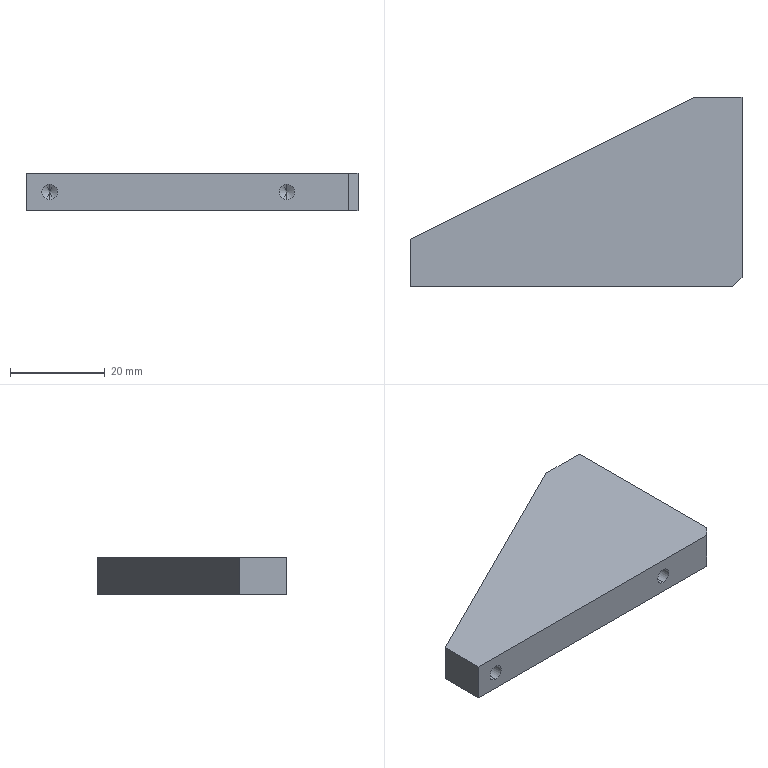Part | SolidWorks | features HoleWzd 2, Chamfer 1, Extrusion 1 | 1 solid | 24 faces | box 70 x 40 x 8 mm | volume 14827 mm3 | cylinder 8 | cone 8 | plane 8 | commonest cylinder face diameters 3.3 x8
STEP:
#1=CARTESIAN_POINT('',(-10.1,35.,5.65));
#2=VERTEX_POINT('',#1);
#3=CARTESIAN_POINT('',(-10.1,35.,2.35));
#4=VERTEX_POINT('',#3);
#5=CARTESIAN_POINT('',(-10.1,35.,4.));
#6=DIRECTION('',(1.,0.,0.));
#7=DIRECTION('',(0.,0.,-1.));
#8=AXIS2_PLACEMENT_3D('',#5,#6,#7);
#9=CIRCLE('',#8,1.65);
#10=EDGE_CURVE('',#2,#4,#9,.T.);
#11=ORIENTED_EDGE('',*,*,#10,.F.);
#12=CARTESIAN_POINT('',(0.,35.,5.65));
#13=VERTEX_POINT('',#12);
#14=CARTESIAN_POINT('',(0.,35.,5.65));
#15=DIRECTION('',(1.,0.,0.));
#16=VECTOR('',#15,1000.);
#17=LINE('',#14,#16);
#18=EDGE_CURVE('',#2,#13,#17,.T.);
#19=ORIENTED_EDGE('',*,*,#18,.T.);
#20=CARTESIAN_POINT('',(0.,35.,2.35));
#21=VERTEX_POINT('',#20);
#22=CARTESIAN_POINT('',(0.,35.,4.));
#23=DIRECTION('',(1.,0.,0.));
#24=DIRECTION('',(0.,0.,-1.));
#25=AXIS2_PLACEMENT_3D('',#22,#23,#24);
#26=CIRCLE('',#25,1.65);
#27=EDGE_CURVE('',#13,#21,#26,.T.);
#28=ORIENTED_EDGE('',*,*,#27,.T.);
#29=CARTESIAN_POINT('',(0.,35.,2.35));
#30=DIRECTION('',(1.,0.,0.));
#31=VECTOR('',#30,1000.);
#32=LINE('',#29,#31);
#33=EDGE_CURVE('',#4,#21,#32,.T.);
#34=ORIENTED_EDGE('',*,*,#33,.F.);
#35=EDGE_LOOP('',(#11,#19,#28,#34));
#36=FACE_OUTER_BOUND('',#35,.T.);
#37=CARTESIAN_POINT('',(0.,35.,4.));
#38=DIRECTION('',(1.,0.,0.));
#39=DIRECTION('',(0.,0.,-1.));
#40=AXIS2_PLACEMENT_3D('',#37,#38,#39);
#41=CYLINDRICAL_SURFACE('',#40,1.65);
#42=ADVANCED_FACE('',(#36),#41,.F.);
#43=CARTESIAN_POINT('',(-11.091,35.,4.));
#44=VERTEX_POINT('',#43);
#45=CARTESIAN_POINT('',(-10.1,35.,2.35));
#46=DIRECTION('',(0.515,0.,-0.8572));
#47=VECTOR('',#46,1000.);
#48=LINE('',#45,#47);
#49=EDGE_CURVE('',#44,#4,#48,.T.);
#50=ORIENTED_EDGE('',*,*,#49,.F.);
#51=CARTESIAN_POINT('',(-10.1,35.,5.65));
#52=DIRECTION('',(0.515,0.,0.8572));
#53=VECTOR('',#52,1000.);
#54=LINE('',#51,#53);
#55=EDGE_CURVE('',#44,#2,#54,.T.);
#56=ORIENTED_EDGE('',*,*,#55,.T.);
#57=ORIENTED_EDGE('',*,*,#10,.T.);
#58=EDGE_LOOP('',(#50,#56,#57));
#59=FACE_OUTER_BOUND('',#58,.T.);
#60=CARTESIAN_POINT('',(-10.1,35.,4.));
#61=DIRECTION('',(1.,0.,0.));
#62=DIRECTION('',(0.,0.,-1.));
#63=AXIS2_PLACEMENT_3D('',#60,#61,#62);
#64=CONICAL_SURFACE('',#63,1.65,1.03);
#65=ADVANCED_FACE('',(#59),#64,.F.);
#66=CARTESIAN_POINT('',(-10.1,15.,5.65));
#67=VERTEX_POINT('',#66);
#68=CARTESIAN_POINT('',(-10.1,15.,2.35));
#69=VERTEX_POINT('',#68);
#70=CARTESIAN_POINT('',(-10.1,15.,4.));
#71=DIRECTION('',(1.,0.,0.));
#72=DIRECTION('',(0.,0.,-1.));
#73=AXIS2_PLACEMENT_3D('',#70,#71,#72);
#74=CIRCLE('',#73,1.65);
#75=EDGE_CURVE('',#67,#69,#74,.T.);
#76=ORIENTED_EDGE('',*,*,#75,.F.);
#77=CARTESIAN_POINT('',(0.,15.,5.65));
#78=VERTEX_POINT('',#77);
#79=CARTESIAN_POINT('',(0.,15.,5.65));
#80=DIRECTION('',(1.,0.,0.));
#81=VECTOR('',#80,1000.);
#82=LINE('',#79,#81);
#83=EDGE_CURVE('',#67,#78,#82,.T.);
#84=ORIENTED_EDGE('',*,*,#83,.T.);
#85=CARTESIAN_POINT('',(0.,15.,2.35));
#86=VERTEX_POINT('',#85);
#87=CARTESIAN_POINT('',(0.,15.,4.));
#88=DIRECTION('',(1.,0.,0.));
#89=DIRECTION('',(0.,0.,-1.));
#90=AXIS2_PLACEMENT_3D('',#87,#88,#89);
#91=CIRCLE('',#90,1.65);
#92=EDGE_CURVE('',#78,#86,#91,.T.);
#93=ORIENTED_EDGE('',*,*,#92,.T.);
#94=CARTESIAN_POINT('',(0.,15.,2.35));
#95=DIRECTION('',(1.,0.,0.));
#96=VECTOR('',#95,1000.);
#97=LINE('',#94,#96);
#98=EDGE_CURVE('',#69,#86,#97,.T.);
#99=ORIENTED_EDGE('',*,*,#98,.F.);
#100=EDGE_LOOP('',(#76,#84,#93,#99));
#101=FACE_OUTER_BOUND('',#100,.T.);
#102=CARTESIAN_POINT('',(0.,15.,4.));
#103=DIRECTION('',(1.,0.,0.));
#104=DIRECTION('',(0.,0.,-1.));
#105=AXIS2_PLACEMENT_3D('',#102,#103,#104);
#106=CYLINDRICAL_SURFACE('',#105,1.65);
#107=ADVANCED_FACE('',(#101),#106,.F.);
#108=CARTESIAN_POINT('',(-11.091,15.,4.));
#109=VERTEX_POINT('',#108);
#110=CARTESIAN_POINT('',(-10.1,15.,2.35));
#111=DIRECTION('',(0.515,0.,-0.8572));
#112=VECTOR('',#111,1000.);
#113=LINE('',#110,#112);
#114=EDGE_CURVE('',#109,#69,#113,.T.);
#115=ORIENTED_EDGE('',*,*,#114,.F.);
#116=CARTESIAN_POINT('',(-10.1,15.,5.65));
#117=DIRECTION('',(0.515,0.,0.8572));
#118=VECTOR('',#117,1000.);
#119=LINE('',#116,#118);
#120=EDGE_CURVE('',#109,#67,#119,.T.);
#121=ORIENTED_EDGE('',*,*,#120,.T.);
#122=ORIENTED_EDGE('',*,*,#75,.T.);
#123=EDGE_LOOP('',(#115,#121,#122));
#124=FACE_OUTER_BOUND('',#123,.T.);
#125=CARTESIAN_POINT('',(-10.1,15.,4.));
#126=DIRECTION('',(1.,0.,0.));
#127=DIRECTION('',(0.,0.,-1.));
#128=AXIS2_PLACEMENT_3D('',#125,#126,#127);
#129=CONICAL_SURFACE('',#128,1.65,1.03);
#130=ADVANCED_FACE('',(#124),#129,.F.);
#131=CARTESIAN_POINT('',(-15.,10.1,5.65));
#132=VERTEX_POINT('',#131);
#133=CARTESIAN_POINT('',(-15.,10.1,2.35));
#134=VERTEX_POINT('',#133);
#135=CARTESIAN_POINT('',(-15.,10.1,4.));
#136=DIRECTION('',(0.,-1.,0.));
#137=DIRECTION('',(0.,0.,-1.));
#138=AXIS2_PLACEMENT_3D('',#135,#136,#137);
#139=CIRCLE('',#138,1.65);
#140=EDGE_CURVE('',#132,#134,#139,.T.);
#141=ORIENTED_EDGE('',*,*,#140,.F.);
#142=CARTESIAN_POINT('',(-15.,0.,5.65));
#143=VERTEX_POINT('',#142);
#144=CARTESIAN_POINT('',(-15.,0.,5.65));
#145=DIRECTION('',(0.,-1.,0.));
#146=VECTOR('',#145,1000.);
#147=LINE('',#144,#146);
#148=EDGE_CURVE('',#132,#143,#147,.T.);
#149=ORIENTED_EDGE('',*,*,#148,.T.);
#150=CARTESIAN_POINT('',(-15.,0.,2.35));
#151=VERTEX_POINT('',#150);
#152=CARTESIAN_POINT('',(-15.,0.,4.));
#153=DIRECTION('',(0.,-1.,0.));
#154=DIRECTION('',(0.,0.,-1.));
#155=AXIS2_PLACEMENT_3D('',#152,#153,#154);
#156=CIRCLE('',#155,1.65);
#157=EDGE_CURVE('',#143,#151,#156,.T.);
#158=ORIENTED_EDGE('',*,*,#157,.T.);
#159=CARTESIAN_POINT('',(-15.,0.,2.35));
#160=DIRECTION('',(0.,-1.,0.));
#161=VECTOR('',#160,1000.);
#162=LINE('',#159,#161);
#163=EDGE_CURVE('',#134,#151,#162,.T.);
#164=ORIENTED_EDGE('',*,*,#163,.F.);
#165=EDGE_LOOP('',(#141,#149,#158,#164));
#166=FACE_OUTER_BOUND('',#165,.T.);
#167=CARTESIAN_POINT('',(-15.,0.,4.));
#168=DIRECTION('',(0.,-1.,0.));
#169=DIRECTION('',(0.,0.,-1.));
#170=AXIS2_PLACEMENT_3D('',#167,#168,#169);
#171=CYLINDRICAL_SURFACE('',#170,1.65);
#172=ADVANCED_FACE('',(#166),#171,.F.);
#173=CARTESIAN_POINT('',(-15.,11.091,4.));
#174=VERTEX_POINT('',#173);
#175=CARTESIAN_POINT('',(-15.,10.1,2.35));
#176=DIRECTION('',(0.,-0.515,-0.8572));
#177=VECTOR('',#176,1000.);
#178=LINE('',#175,#177);
#179=EDGE_CURVE('',#174,#134,#178,.T.);
#180=ORIENTED_EDGE('',*,*,#179,.F.);
#181=CARTESIAN_POINT('',(-15.,10.1,5.65));
#182=DIRECTION('',(0.,-0.515,0.8572));
#183=VECTOR('',#182,1000.);
#184=LINE('',#181,#183);
#185=EDGE_CURVE('',#174,#132,#184,.T.);
#186=ORIENTED_EDGE('',*,*,#185,.T.);
#187=ORIENTED_EDGE('',*,*,#140,.T.);
#188=EDGE_LOOP('',(#180,#186,#187));
#189=FACE_OUTER_BOUND('',#188,.T.);
#190=CARTESIAN_POINT('',(-15.,10.1,4.));
#191=DIRECTION('',(0.,-1.,0.));
#192=DIRECTION('',(0.,0.,-1.));
#193=AXIS2_PLACEMENT_3D('',#190,#191,#192);
#194=CONICAL_SURFACE('',#193,1.65,1.03);
#195=ADVANCED_FACE('',(#189),#194,.F.);
#196=CARTESIAN_POINT('',(-65.,10.1,5.65));
#197=VERTEX_POINT('',#196);
#198=CARTESIAN_POINT('',(-65.,10.1,2.35));
#199=VERTEX_POINT('',#198);
#200=CARTESIAN_POINT('',(-65.,10.1,4.));
#201=DIRECTION('',(0.,-1.,0.));
#202=DIRECTION('',(0.,0.,-1.));
#203=AXIS2_PLACEMENT_3D('',#200,#201,#202);
#204=CIRCLE('',#203,1.65);
#205=EDGE_CURVE('',#197,#199,#204,.T.);
#206=ORIENTED_EDGE('',*,*,#205,.F.);
#207=CARTESIAN_POINT('',(-65.,0.,5.65));
#208=VERTEX_POINT('',#207);
#209=CARTESIAN_POINT('',(-65.,0.,5.65));
#210=DIRECTION('',(0.,-1.,0.));
#211=VECTOR('',#210,1000.);
#212=LINE('',#209,#211);
#213=EDGE_CURVE('',#197,#208,#212,.T.);
#214=ORIENTED_EDGE('',*,*,#213,.T.);
#215=CARTESIAN_POINT('',(-65.,0.,2.35));
#216=VERTEX_POINT('',#215);
#217=CARTESIAN_POINT('',(-65.,0.,4.));
#218=DIRECTION('',(0.,-1.,0.));
#219=DIRECTION('',(0.,0.,-1.));
#220=AXIS2_PLACEMENT_3D('',#217,#218,#219);
#221=CIRCLE('',#220,1.65);
#222=EDGE_CURVE('',#208,#216,#221,.T.);
#223=ORIENTED_EDGE('',*,*,#222,.T.);
#224=CARTESIAN_POINT('',(-65.,0.,2.35));
#225=DIRECTION('',(0.,-1.,0.));
#226=VECTOR('',#225,1000.);
#227=LINE('',#224,#226);
#228=EDGE_CURVE('',#199,#216,#227,.T.);
#229=ORIENTED_EDGE('',*,*,#228,.F.);
#230=EDGE_LOOP('',(#206,#214,#223,#229));
#231=FACE_OUTER_BOUND('',#230,.T.);
#232=CARTESIAN_POINT('',(-65.,0.,4.));
#233=DIRECTION('',(0.,-1.,0.));
#234=DIRECTION('',(0.,0.,-1.));
#235=AXIS2_PLACEMENT_3D('',#232,#233,#234);
#236=CYLINDRICAL_SURFACE('',#235,1.65);
#237=ADVANCED_FACE('',(#231),#236,.F.);
#238=CARTESIAN_POINT('',(-65.,11.091,4.));
#239=VERTEX_POINT('',#238);
#240=CARTESIAN_POINT('',(-65.,10.1,2.35));
#241=DIRECTION('',(0.,-0.515,-0.8572));
#242=VECTOR('',#241,1000.);
#243=LINE('',#240,#242);
#244=EDGE_CURVE('',#239,#199,#243,.T.);
#245=ORIENTED_EDGE('',*,*,#244,.F.);
#246=CARTESIAN_POINT('',(-65.,10.1,5.65));
#247=DIRECTION('',(0.,-0.515,0.8572));
#248=VECTOR('',#247,1000.);
#249=LINE('',#246,#248);
#250=EDGE_CURVE('',#239,#197,#249,.T.);
#251=ORIENTED_EDGE('',*,*,#250,.T.);
#252=ORIENTED_EDGE('',*,*,#205,.T.);
#253=EDGE_LOOP('',(#245,#251,#252));
#254=FACE_OUTER_BOUND('',#253,.T.);
#255=CARTESIAN_POINT('',(-65.,10.1,4.));
#256=DIRECTION('',(0.,-1.,0.));
#257=DIRECTION('',(0.,0.,-1.));
#258=AXIS2_PLACEMENT_3D('',#255,#256,#257);
#259=CONICAL_SURFACE('',#258,1.65,1.03);
#260=ADVANCED_FACE('',(#254),#259,.F.);
#261=CARTESIAN_POINT('',(-15.,0.,4.));
#262=DIRECTION('',(0.,-1.,0.));
#263=DIRECTION('',(0.,0.,-1.));
#264=AXIS2_PLACEMENT_3D('',#261,#262,#263);
#265=CIRCLE('',#264,1.65);
#266=EDGE_CURVE('',#151,#143,#265,.T.);
#267=ORIENTED_EDGE('',*,*,#266,.F.);
#268=ORIENTED_EDGE('',*,*,#157,.F.);
#269=EDGE_LOOP('',(#267,#268));
#270=FACE_BOUND('',#269,.T.);
#271=CARTESIAN_POINT('',(-65.,0.,4.));
#272=DIRECTION('',(0.,-1.,0.));
#273=DIRECTION('',(0.,0.,-1.));
#274=AXIS2_PLACEMENT_3D('',#271,#272,#273);
#275=CIRCLE('',#274,1.65);
#276=EDGE_CURVE('',#216,#208,#275,.T.);
#277=ORIENTED_EDGE('',*,*,#276,.F.);
#278=ORIENTED_EDGE('',*,*,#222,.F.);
#279=EDGE_LOOP('',(#277,#278));
#280=FACE_BOUND('',#279,.T.);
#281=CARTESIAN_POINT('',(-70.,0.,0.));
#282=VERTEX_POINT('',#281);
#283=CARTESIAN_POINT('',(-2.,0.,0.));
#284=VERTEX_POINT('',#283);
#285=CARTESIAN_POINT('',(-70.,0.,0.));
#286=DIRECTION('',(1.,0.,0.));
#287=VECTOR('',#286,1000.);
#288=LINE('',#285,#287);
#289=EDGE_CURVE('',#282,#284,#288,.T.);
#290=ORIENTED_EDGE('',*,*,#289,.T.);
#291=CARTESIAN_POINT('',(-2.,0.,8.));
#292=VERTEX_POINT('',#291);
#293=CARTESIAN_POINT('',(-2.,0.,8.));
#294=DIRECTION('',(0.,0.,1.));
#295=VECTOR('',#294,1000.);
#296=LINE('',#293,#295);
#297=EDGE_CURVE('',#284,#292,#296,.T.);
#298=ORIENTED_EDGE('',*,*,#297,.T.);
#299=CARTESIAN_POINT('',(-70.,0.,8.));
#300=VERTEX_POINT('',#299);
#301=CARTESIAN_POINT('',(-70.,0.,8.));
#302=DIRECTION('',(1.,0.,0.));
#303=VECTOR('',#302,1000.);
#304=LINE('',#301,#303);
#305=EDGE_CURVE('',#300,#292,#304,.T.);
#306=ORIENTED_EDGE('',*,*,#305,.F.);
#307=CARTESIAN_POINT('',(-70.,0.,8.));
#308=DIRECTION('',(0.,0.,-1.));
#309=VECTOR('',#308,1000.);
#310=LINE('',#307,#309);
#311=EDGE_CURVE('',#300,#282,#310,.T.);
#312=ORIENTED_EDGE('',*,*,#311,.T.);
#313=EDGE_LOOP('',(#290,#298,#306,#312));
#314=FACE_OUTER_BOUND('',#313,.T.);
#315=CARTESIAN_POINT('',(-70.,0.,8.));
#316=DIRECTION('',(0.,1.,0.));
#317=DIRECTION('',(0.,0.,1.));
#318=AXIS2_PLACEMENT_3D('',#315,#316,#317);
#319=PLANE('',#318);
#320=ADVANCED_FACE('',(#270,#280,#314),#319,.F.);
#321=CARTESIAN_POINT('',(0.,35.,4.));
#322=DIRECTION('',(1.,0.,0.));
#323=DIRECTION('',(0.,0.,-1.));
#324=AXIS2_PLACEMENT_3D('',#321,#322,#323);
#325=CIRCLE('',#324,1.65);
#326=EDGE_CURVE('',#21,#13,#325,.T.);
#327=ORIENTED_EDGE('',*,*,#326,.F.);
#328=ORIENTED_EDGE('',*,*,#27,.F.);
#329=EDGE_LOOP('',(#327,#328));
#330=FACE_BOUND('',#329,.T.);
#331=CARTESIAN_POINT('',(0.,15.,4.));
#332=DIRECTION('',(1.,0.,0.));
#333=DIRECTION('',(0.,0.,-1.));
#334=AXIS2_PLACEMENT_3D('',#331,#332,#333);
#335=CIRCLE('',#334,1.65);
#336=EDGE_CURVE('',#86,#78,#335,.T.);
#337=ORIENTED_EDGE('',*,*,#336,.F.);
#338=ORIENTED_EDGE('',*,*,#92,.F.);
#339=EDGE_LOOP('',(#337,#338));
#340=FACE_BOUND('',#339,.T.);
#341=CARTESIAN_POINT('',(0.,2.,8.));
#342=VERTEX_POINT('',#341);
#343=CARTESIAN_POINT('',(0.,40.,8.));
#344=VERTEX_POINT('',#343);
#345=CARTESIAN_POINT('',(0.,0.,8.));
#346=DIRECTION('',(0.,1.,0.));
#347=VECTOR('',#346,1000.);
#348=LINE('',#345,#347);
#349=EDGE_CURVE('',#342,#344,#348,.T.);
#350=ORIENTED_EDGE('',*,*,#349,.F.);
#351=CARTESIAN_POINT('',(0.,2.,0.));
#352=VERTEX_POINT('',#351);
#353=CARTESIAN_POINT('',(0.,2.,8.));
#354=DIRECTION('',(0.,0.,-1.));
#355=VECTOR('',#354,1000.);
#356=LINE('',#353,#355);
#357=EDGE_CURVE('',#342,#352,#356,.T.);
#358=ORIENTED_EDGE('',*,*,#357,.T.);
#359=CARTESIAN_POINT('',(0.,40.,0.));
#360=VERTEX_POINT('',#359);
#361=CARTESIAN_POINT('',(0.,0.,0.));
#362=DIRECTION('',(0.,1.,0.));
#363=VECTOR('',#362,1000.);
#364=LINE('',#361,#363);
#365=EDGE_CURVE('',#352,#360,#364,.T.);
#366=ORIENTED_EDGE('',*,*,#365,.T.);
#367=CARTESIAN_POINT('',(0.,40.,8.));
#368=DIRECTION('',(0.,0.,-1.));
#369=VECTOR('',#368,1000.);
#370=LINE('',#367,#369);
#371=EDGE_CURVE('',#344,#360,#370,.T.);
#372=ORIENTED_EDGE('',*,*,#371,.F.);
#373=EDGE_LOOP('',(#350,#358,#366,#372));
#374=FACE_OUTER_BOUND('',#373,.T.);
#375=CARTESIAN_POINT('',(0.,0.,8.));
#376=DIRECTION('',(-1.,0.,0.));
#377=DIRECTION('',(0.,0.,1.));
#378=AXIS2_PLACEMENT_3D('',#375,#376,#377);
#379=PLANE('',#378);
#380=ADVANCED_FACE('',(#330,#340,#374),#379,.F.);
#381=CARTESIAN_POINT('',(-10.,40.,0.));
#382=VERTEX_POINT('',#381);
#383=CARTESIAN_POINT('',(0.,40.,0.));
#384=DIRECTION('',(-1.,0.,0.));
#385=VECTOR('',#384,1000.);
#386=LINE('',#383,#385);
#387=EDGE_CURVE('',#360,#382,#386,.T.);
#388=ORIENTED_EDGE('',*,*,#387,.T.);
#389=CARTESIAN_POINT('',(-10.,40.,8.));
#390=VERTEX_POINT('',#389);
#391=CARTESIAN_POINT('',(-10.,40.,8.));
#392=DIRECTION('',(0.,0.,-1.));
#393=VECTOR('',#392,1000.);
#394=LINE('',#391,#393);
#395=EDGE_CURVE('',#390,#382,#394,.T.);
#396=ORIENTED_EDGE('',*,*,#395,.F.);
#397=CARTESIAN_POINT('',(0.,40.,8.));
#398=DIRECTION('',(-1.,0.,0.));
#399=VECTOR('',#398,1000.);
#400=LINE('',#397,#399);
#401=EDGE_CURVE('',#344,#390,#400,.T.);
#402=ORIENTED_EDGE('',*,*,#401,.F.);
#403=ORIENTED_EDGE('',*,*,#371,.T.);
#404=EDGE_LOOP('',(#388,#396,#402,#403));
#405=FACE_OUTER_BOUND('',#404,.T.);
#406=CARTESIAN_POINT('',(0.,40.,8.));
#407=DIRECTION('',(0.,-1.,0.));
#408=DIRECTION('',(0.,0.,-1.));
#409=AXIS2_PLACEMENT_3D('',#406,#407,#408);
#410=PLANE('',#409);
#411=ADVANCED_FACE('',(#405),#410,.F.);
#412=CARTESIAN_POINT('',(-70.,10.,0.));
#413=VERTEX_POINT('',#412);
#414=CARTESIAN_POINT('',(-10.,40.,0.));
#415=DIRECTION('',(-0.8944,-0.4472,0.));
#416=VECTOR('',#415,1000.);
#417=LINE('',#414,#416);
#418=EDGE_CURVE('',#382,#413,#417,.T.);
#419=ORIENTED_EDGE('',*,*,#418,.T.);
#420=CARTESIAN_POINT('',(-70.,10.,8.));
#421=VERTEX_POINT('',#420);
#422=CARTESIAN_POINT('',(-70.,10.,8.));
#423=DIRECTION('',(0.,0.,-1.));
#424=VECTOR('',#423,1000.);
#425=LINE('',#422,#424);
#426=EDGE_CURVE('',#421,#413,#425,.T.);
#427=ORIENTED_EDGE('',*,*,#426,.F.);
#428=CARTESIAN_POINT('',(-10.,40.,8.));
#429=DIRECTION('',(-0.8944,-0.4472,0.));
#430=VECTOR('',#429,1000.);
#431=LINE('',#428,#430);
#432=EDGE_CURVE('',#390,#421,#431,.T.);
#433=ORIENTED_EDGE('',*,*,#432,.F.);
#434=ORIENTED_EDGE('',*,*,#395,.T.);
#435=EDGE_LOOP('',(#419,#427,#433,#434));
#436=FACE_OUTER_BOUND('',#435,.T.);
#437=CARTESIAN_POINT('',(-10.,40.,8.));
#438=DIRECTION('',(0.4472,-0.8944,0.));
#439=DIRECTION('',(0.8944,0.4472,0.));
#440=AXIS2_PLACEMENT_3D('',#437,#438,#439);
#441=PLANE('',#440);
#442=ADVANCED_FACE('',(#436),#441,.F.);
#443=CARTESIAN_POINT('',(-70.,10.,0.));
#444=DIRECTION('',(0.,-1.,0.));
#445=VECTOR('',#444,1000.);
#446=LINE('',#443,#445);
#447=EDGE_CURVE('',#413,#282,#446,.T.);
#448=ORIENTED_EDGE('',*,*,#447,.T.);
#449=ORIENTED_EDGE('',*,*,#311,.F.);
#450=CARTESIAN_POINT('',(-70.,10.,8.));
#451=DIRECTION('',(0.,-1.,0.));
#452=VECTOR('',#451,1000.);
#453=LINE('',#450,#452);
#454=EDGE_CURVE('',#421,#300,#453,.T.);
#455=ORIENTED_EDGE('',*,*,#454,.F.);
#456=ORIENTED_EDGE('',*,*,#426,.T.);
#457=EDGE_LOOP('',(#448,#449,#455,#456));
#458=FACE_OUTER_BOUND('',#457,.T.);
#459=CARTESIAN_POINT('',(-70.,10.,8.));
#460=DIRECTION('',(1.,0.,0.));
#461=DIRECTION('',(0.,0.,-1.));
#462=AXIS2_PLACEMENT_3D('',#459,#460,#461);
#463=PLANE('',#462);
#464=ADVANCED_FACE('',(#458),#463,.F.);
#465=ORIENTED_EDGE('',*,*,#305,.T.);
#466=CARTESIAN_POINT('',(-1.,1.,8.));
#467=DIRECTION('',(0.7071,0.7071,0.));
#468=VECTOR('',#467,1000.);
#469=LINE('',#466,#468);
#470=EDGE_CURVE('',#292,#342,#469,.T.);
#471=ORIENTED_EDGE('',*,*,#470,.T.);
#472=ORIENTED_EDGE('',*,*,#349,.T.);
#473=ORIENTED_EDGE('',*,*,#401,.T.);
#474=ORIENTED_EDGE('',*,*,#432,.T.);
#475=ORIENTED_EDGE('',*,*,#454,.T.);
#476=EDGE_LOOP('',(#465,#471,#472,#473,#474,#475));
#477=FACE_OUTER_BOUND('',#476,.T.);
#478=CARTESIAN_POINT('',(0.,0.,8.));
#479=DIRECTION('',(0.,0.,1.));
#480=DIRECTION('',(1.,0.,0.));
#481=AXIS2_PLACEMENT_3D('',#478,#479,#480);
#482=PLANE('',#481);
#483=ADVANCED_FACE('',(#477),#482,.T.);
#484=ORIENTED_EDGE('',*,*,#365,.F.);
#485=CARTESIAN_POINT('',(0.,2.,0.));
#486=DIRECTION('',(-0.7071,-0.7071,0.));
#487=VECTOR('',#486,1000.);
#488=LINE('',#485,#487);
#489=EDGE_CURVE('',#352,#284,#488,.T.);
#490=ORIENTED_EDGE('',*,*,#489,.T.);
#491=ORIENTED_EDGE('',*,*,#289,.F.);
#492=ORIENTED_EDGE('',*,*,#447,.F.);
#493=ORIENTED_EDGE('',*,*,#418,.F.);
#494=ORIENTED_EDGE('',*,*,#387,.F.);
#495=EDGE_LOOP('',(#484,#490,#491,#492,#493,#494));
#496=FACE_OUTER_BOUND('',#495,.T.);
#497=CARTESIAN_POINT('',(0.,0.,0.));
#498=DIRECTION('',(0.,0.,1.));
#499=DIRECTION('',(1.,0.,0.));
#500=AXIS2_PLACEMENT_3D('',#497,#498,#499);
#501=PLANE('',#500);
#502=ADVANCED_FACE('',(#496),#501,.F.);
#503=ORIENTED_EDGE('',*,*,#250,.F.);
#504=ORIENTED_EDGE('',*,*,#244,.T.);
#505=CARTESIAN_POINT('',(-65.,10.1,4.));
#506=DIRECTION('',(0.,-1.,0.));
#507=DIRECTION('',(0.,0.,-1.));
#508=AXIS2_PLACEMENT_3D('',#505,#506,#507);
#509=CIRCLE('',#508,1.65);
#510=EDGE_CURVE('',#199,#197,#509,.T.);
#511=ORIENTED_EDGE('',*,*,#510,.T.);
#512=EDGE_LOOP('',(#503,#504,#511));
#513=FACE_OUTER_BOUND('',#512,.T.);
#514=CARTESIAN_POINT('',(-65.,10.1,4.));
#515=DIRECTION('',(0.,-1.,0.));
#516=DIRECTION('',(0.,0.,-1.));
#517=AXIS2_PLACEMENT_3D('',#514,#515,#516);
#518=CONICAL_SURFACE('',#517,1.65,1.03);
#519=ADVANCED_FACE('',(#513),#518,.F.);
#520=ORIENTED_EDGE('',*,*,#213,.F.);
#521=ORIENTED_EDGE('',*,*,#510,.F.);
#522=ORIENTED_EDGE('',*,*,#228,.T.);
#523=ORIENTED_EDGE('',*,*,#276,.T.);
#524=EDGE_LOOP('',(#520,#521,#522,#523));
#525=FACE_OUTER_BOUND('',#524,.T.);
#526=CARTESIAN_POINT('',(-65.,0.,4.));
#527=DIRECTION('',(0.,-1.,0.));
#528=DIRECTION('',(0.,0.,-1.));
#529=AXIS2_PLACEMENT_3D('',#526,#527,#528);
#530=CYLINDRICAL_SURFACE('',#529,1.65);
#531=ADVANCED_FACE('',(#525),#530,.F.);
#532=ORIENTED_EDGE('',*,*,#185,.F.);
#533=ORIENTED_EDGE('',*,*,#179,.T.);
#534=CARTESIAN_POINT('',(-15.,10.1,4.));
#535=DIRECTION('',(0.,-1.,0.));
#536=DIRECTION('',(0.,0.,-1.));
#537=AXIS2_PLACEMENT_3D('',#534,#535,#536);
#538=CIRCLE('',#537,1.65);
#539=EDGE_CURVE('',#134,#132,#538,.T.);
#540=ORIENTED_EDGE('',*,*,#539,.T.);
#541=EDGE_LOOP('',(#532,#533,#540));
#542=FACE_OUTER_BOUND('',#541,.T.);
#543=CARTESIAN_POINT('',(-15.,10.1,4.));
#544=DIRECTION('',(0.,-1.,0.));
#545=DIRECTION('',(0.,0.,-1.));
#546=AXIS2_PLACEMENT_3D('',#543,#544,#545);
#547=CONICAL_SURFACE('',#546,1.65,1.03);
#548=ADVANCED_FACE('',(#542),#547,.F.);
#549=ORIENTED_EDGE('',*,*,#148,.F.);
#550=ORIENTED_EDGE('',*,*,#539,.F.);
#551=ORIENTED_EDGE('',*,*,#163,.T.);
#552=ORIENTED_EDGE('',*,*,#266,.T.);
#553=EDGE_LOOP('',(#549,#550,#551,#552));
#554=FACE_OUTER_BOUND('',#553,.T.);
#555=CARTESIAN_POINT('',(-15.,0.,4.));
#556=DIRECTION('',(0.,-1.,0.));
#557=DIRECTION('',(0.,0.,-1.));
#558=AXIS2_PLACEMENT_3D('',#555,#556,#557);
#559=CYLINDRICAL_SURFACE('',#558,1.65);
#560=ADVANCED_FACE('',(#554),#559,.F.);
#561=ORIENTED_EDGE('',*,*,#120,.F.);
#562=ORIENTED_EDGE('',*,*,#114,.T.);
#563=CARTESIAN_POINT('',(-10.1,15.,4.));
#564=DIRECTION('',(1.,0.,0.));
#565=DIRECTION('',(0.,0.,-1.));
#566=AXIS2_PLACEMENT_3D('',#563,#564,#565);
#567=CIRCLE('',#566,1.65);
#568=EDGE_CURVE('',#69,#67,#567,.T.);
#569=ORIENTED_EDGE('',*,*,#568,.T.);
#570=EDGE_LOOP('',(#561,#562,#569));
#571=FACE_OUTER_BOUND('',#570,.T.);
#572=CARTESIAN_POINT('',(-10.1,15.,4.));
#573=DIRECTION('',(1.,0.,0.));
#574=DIRECTION('',(0.,0.,-1.));
#575=AXIS2_PLACEMENT_3D('',#572,#573,#574);
#576=CONICAL_SURFACE('',#575,1.65,1.03);
#577=ADVANCED_FACE('',(#571),#576,.F.);
#578=ORIENTED_EDGE('',*,*,#83,.F.);
#579=ORIENTED_EDGE('',*,*,#568,.F.);
#580=ORIENTED_EDGE('',*,*,#98,.T.);
#581=ORIENTED_EDGE('',*,*,#336,.T.);
#582=EDGE_LOOP('',(#578,#579,#580,#581));
#583=FACE_OUTER_BOUND('',#582,.T.);
#584=CARTESIAN_POINT('',(0.,15.,4.));
#585=DIRECTION('',(1.,0.,0.));
#586=DIRECTION('',(0.,0.,-1.));
#587=AXIS2_PLACEMENT_3D('',#584,#585,#586);
#588=CYLINDRICAL_SURFACE('',#587,1.65);
#589=ADVANCED_FACE('',(#583),#588,.F.);
#590=ORIENTED_EDGE('',*,*,#55,.F.);
#591=ORIENTED_EDGE('',*,*,#49,.T.);
#592=CARTESIAN_POINT('',(-10.1,35.,4.));
#593=DIRECTION('',(1.,0.,0.));
#594=DIRECTION('',(0.,0.,-1.));
#595=AXIS2_PLACEMENT_3D('',#592,#593,#594);
#596=CIRCLE('',#595,1.65);
#597=EDGE_CURVE('',#4,#2,#596,.T.);
#598=ORIENTED_EDGE('',*,*,#597,.T.);
#599=EDGE_LOOP('',(#590,#591,#598));
#600=FACE_OUTER_BOUND('',#599,.T.);
#601=CARTESIAN_POINT('',(-10.1,35.,4.));
#602=DIRECTION('',(1.,0.,0.));
#603=DIRECTION('',(0.,0.,-1.));
#604=AXIS2_PLACEMENT_3D('',#601,#602,#603);
#605=CONICAL_SURFACE('',#604,1.65,1.03);
#606=ADVANCED_FACE('',(#600),#605,.F.);
#607=ORIENTED_EDGE('',*,*,#18,.F.);
#608=ORIENTED_EDGE('',*,*,#597,.F.);
#609=ORIENTED_EDGE('',*,*,#33,.T.);
#610=ORIENTED_EDGE('',*,*,#326,.T.);
#611=EDGE_LOOP('',(#607,#608,#609,#610));
#612=FACE_OUTER_BOUND('',#611,.T.);
#613=CARTESIAN_POINT('',(0.,35.,4.));
#614=DIRECTION('',(1.,0.,0.));
#615=DIRECTION('',(0.,0.,-1.));
#616=AXIS2_PLACEMENT_3D('',#613,#614,#615);
#617=CYLINDRICAL_SURFACE('',#616,1.65);
#618=ADVANCED_FACE('',(#612),#617,.F.);
#619=ORIENTED_EDGE('',*,*,#470,.F.);
#620=ORIENTED_EDGE('',*,*,#297,.F.);
#621=ORIENTED_EDGE('',*,*,#489,.F.);
#622=ORIENTED_EDGE('',*,*,#357,.F.);
#623=EDGE_LOOP('',(#619,#620,#621,#622));
#624=FACE_OUTER_BOUND('',#623,.T.);
#625=CARTESIAN_POINT('',(0.,2.,8.));
#626=DIRECTION('',(-0.7071,0.7071,0.));
#627=DIRECTION('',(0.,0.,-1.));
#628=AXIS2_PLACEMENT_3D('',#625,#626,#627);
#629=PLANE('',#628);
#630=ADVANCED_FACE('',(#624),#629,.F.);
#631=CLOSED_SHELL('',(#42,#65,#107,#130,#172,#195,#237,#260,#320,#380,#411,#442,#464,#483,#502,#519,#531,#548,#560,#577,#589,#606,#618,#630));
#632=MANIFOLD_SOLID_BREP('',#631);
#633=CARTESIAN_POINT('',(0.,0.,0.));
#634=DIRECTION('',(0.,0.,1.));
#635=DIRECTION('',(1.,0.,0.));
#636=AXIS2_PLACEMENT_3D('',#633,#634,#635);
#637=(LENGTH_UNIT()NAMED_UNIT(*)SI_UNIT(.MILLI.,.METRE.));
#638=UNCERTAINTY_MEASURE_WITH_UNIT(LENGTH_MEASURE(0.00001),#637,'','');
#639=(NAMED_UNIT(*)PLANE_ANGLE_UNIT()SI_UNIT($,.RADIAN.));
#640=(NAMED_UNIT(*)SI_UNIT($,.STERADIAN.)SOLID_ANGLE_UNIT());
#641=(GEOMETRIC_REPRESENTATION_CONTEXT(3)GLOBAL_UNCERTAINTY_ASSIGNED_CONTEXT((#638))GLOBAL_UNIT_ASSIGNED_CONTEXT((#637,#639,#640))REPRESENTATION_CONTEXT('',''));
#642=ADVANCED_BREP_SHAPE_REPRESENTATION('',(#632,#636),#641);